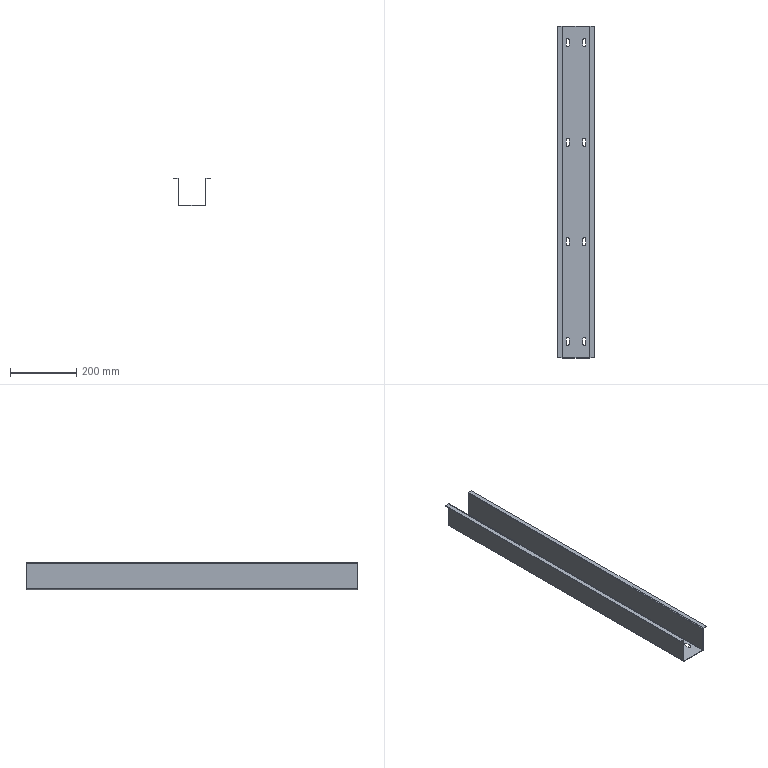Part | SolidWorks | features BaseBody 1 | 1 solid | 70 faces | box 110 x 1000 x 81.5 mm | volume 399038 mm3 | plane 46 | cylinder 24 | commonest cylinder face diameters 10 x16 1 x4 4 x4